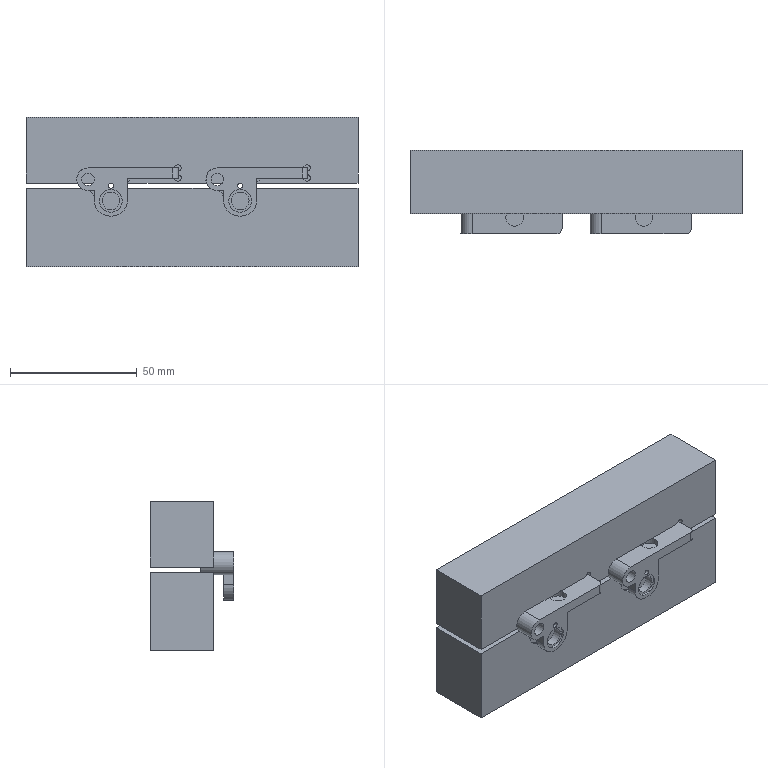Part | 4 solids | 118 faces | box 131 x 33 x 59 mm | volume 189481 mm3 | plane 64 | cylinder 54 | commonest cylinder face diameters 12 x12 9 x10 6 x8 7 x6 2 x4 2.05 x4